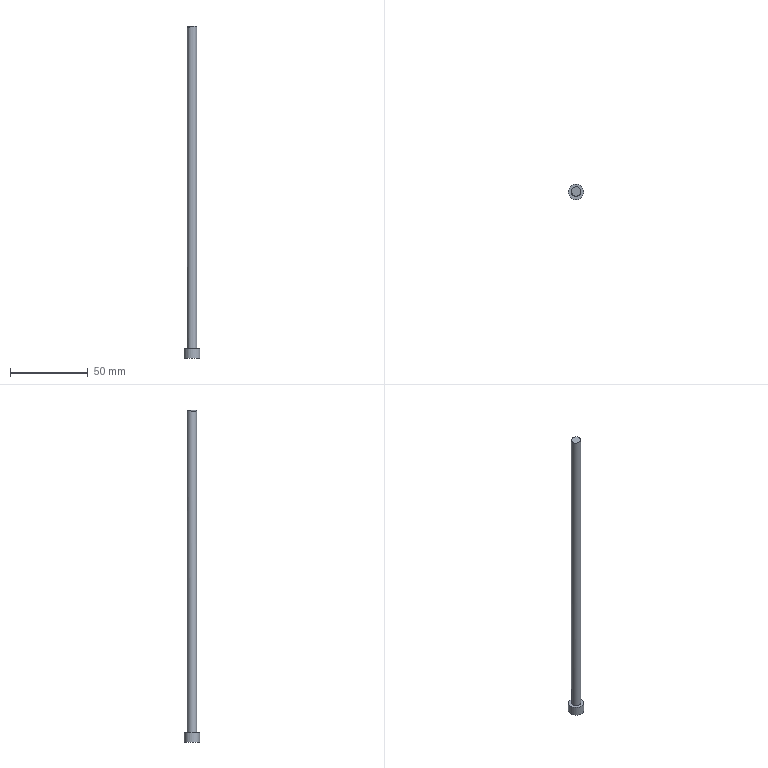Part | NX | features DDZ6.00 2 | 1 solid | 5 faces | box 10 x 10 x 214.007 mm | volume 6341 mm3 | cylinder 2 | plane 2 | sphere 1 | commonest cylinder face diameters 6 x1 10 x1
STEP:
#1=CARTESIAN_POINT('',(-27.91,-12.97,-204.5));
#2=VERTEX_POINT('',#1);
#3=CARTESIAN_POINT('',(-30.91,-12.97,-204.5));
#4=DIRECTION('',(0.,0.,1.));
#5=DIRECTION('',(1.,0.,0.));
#6=AXIS2_PLACEMENT_3D('',#3,#4,#5);
#7=CIRCLE('',#6,3.);
#8=EDGE_CURVE('',#2,#2,#7,.F.);
#9=ORIENTED_EDGE('',*,*,#8,.F.);
#10=EDGE_LOOP('',(#9));
#11=FACE_BOUND('',#10,.T.);
#12=CARTESIAN_POINT('',(-33.046,-15.077,2.797));
#13=VERTEX_POINT('',#12);
#14=CARTESIAN_POINT('',(-30.927,-16.293,2.98));
#15=CARTESIAN_POINT('',(-33.278,-15.308,2.76));
#16=CARTESIAN_POINT('',(-34.236,-12.935,2.764));
#17=CARTESIAN_POINT('',(-33.236,-10.599,2.989));
#18=CARTESIAN_POINT('',(-30.891,-9.647,3.3));
#19=CARTESIAN_POINT('',(-28.544,-10.632,3.519));
#20=CARTESIAN_POINT('',(-27.583,-13.,3.515));
#21=CARTESIAN_POINT('',(-28.583,-15.341,3.291));
#22=CARTESIAN_POINT('',(-30.927,-16.293,2.98));
#23=CARTESIAN_POINT('',(-33.278,-15.308,2.76));
#24=CARTESIAN_POINT('',(-34.236,-12.935,2.764));
#25=B_SPLINE_CURVE_WITH_KNOTS('',3,(#14,#15,#16,#17,#18,#19,#20,#21,#22,#23,#24),.UNSPECIFIED.,.T.,.F.,(1,1,1,1,1,1,1,1,1,1,1,1,1,1,1),(-0.007061,-0.004707,-0.002354,0.,0.002354,0.004707,0.007061,0.009414,0.01177,0.01412,0.01648,0.01883,0.02118,0.02354,0.02589),.UNSPECIFIED.);
#26=EDGE_CURVE('',#13,#13,#25,.T.);
#27=ORIENTED_EDGE('',*,*,#26,.T.);
#28=EDGE_LOOP('',(#27));
#29=FACE_BOUND('',#28,.T.);
#30=CARTESIAN_POINT('',(-30.91,-12.97,-210.5));
#31=DIRECTION('',(0.,0.,1.));
#32=DIRECTION('',(1.,0.,0.));
#33=AXIS2_PLACEMENT_3D('',#30,#31,#32);
#34=CYLINDRICAL_SURFACE('',#33,3.);
#35=ADVANCED_FACE('',(#11,#29),#34,.T.);
#36=ORIENTED_EDGE('',*,*,#8,.T.);
#37=EDGE_LOOP('',(#36));
#38=FACE_BOUND('',#37,.T.);
#39=CARTESIAN_POINT('',(-25.91,-12.97,-204.5));
#40=VERTEX_POINT('',#39);
#41=CARTESIAN_POINT('',(-30.91,-12.97,-204.5));
#42=DIRECTION('',(0.,0.,-1.));
#43=DIRECTION('',(1.,0.,0.));
#44=AXIS2_PLACEMENT_3D('',#41,#42,#43);
#45=CIRCLE('',#44,5.);
#46=EDGE_CURVE('',#40,#40,#45,.T.);
#47=ORIENTED_EDGE('',*,*,#46,.F.);
#48=EDGE_LOOP('',(#47));
#49=FACE_BOUND('',#48,.T.);
#50=CARTESIAN_POINT('',(-30.91,-12.97,-204.5));
#51=DIRECTION('',(0.,0.,1.));
#52=DIRECTION('',(1.,0.,0.));
#53=AXIS2_PLACEMENT_3D('',#50,#51,#52);
#54=PLANE('',#53);
#55=ADVANCED_FACE('',(#38,#49),#54,.T.);
#56=ORIENTED_EDGE('',*,*,#46,.T.);
#57=EDGE_LOOP('',(#56));
#58=FACE_BOUND('',#57,.T.);
#59=CARTESIAN_POINT('',(-25.91,-12.97,-210.5));
#60=VERTEX_POINT('',#59);
#61=CARTESIAN_POINT('',(-30.91,-12.97,-210.5));
#62=DIRECTION('',(0.,0.,1.));
#63=DIRECTION('',(1.,0.,0.));
#64=AXIS2_PLACEMENT_3D('',#61,#62,#63);
#65=CIRCLE('',#64,5.);
#66=EDGE_CURVE('',#60,#60,#65,.T.);
#67=ORIENTED_EDGE('',*,*,#66,.T.);
#68=EDGE_LOOP('',(#67));
#69=FACE_BOUND('',#68,.T.);
#70=CARTESIAN_POINT('',(-30.91,-12.97,-210.5));
#71=DIRECTION('',(0.,0.,1.));
#72=DIRECTION('',(1.,0.,0.));
#73=AXIS2_PLACEMENT_3D('',#70,#71,#72);
#74=CYLINDRICAL_SURFACE('',#73,5.);
#75=ADVANCED_FACE('',(#58,#69),#74,.T.);
#76=ORIENTED_EDGE('',*,*,#66,.F.);
#77=EDGE_LOOP('',(#76));
#78=FACE_BOUND('',#77,.T.);
#79=CARTESIAN_POINT('',(-30.91,-12.97,-210.5));
#80=DIRECTION('',(0.,0.,-1.));
#81=DIRECTION('',(-1.,0.,0.));
#82=AXIS2_PLACEMENT_3D('',#79,#80,#81);
#83=PLANE('',#82);
#84=ADVANCED_FACE('',(#78),#83,.T.);
#85=ORIENTED_EDGE('',*,*,#26,.F.);
#86=EDGE_LOOP('',(#85));
#87=FACE_BOUND('',#86,.T.);
#88=CARTESIAN_POINT('',(0.,0.,-269.66));
#89=DIRECTION('',(0.,0.,-1.));
#90=DIRECTION('',(1.,0.,0.));
#91=AXIS2_PLACEMENT_3D('',#88,#89,#90);
#92=SPHERICAL_SURFACE('',#91,274.868);
#93=ADVANCED_FACE('',(#87),#92,.T.);
#94=CLOSED_SHELL('',(#35,#55,#75,#84,#93));
#95=MANIFOLD_SOLID_BREP('',#94);
#96=(LENGTH_UNIT()NAMED_UNIT(*)SI_UNIT(.MILLI.,.METRE.));
#97=UNCERTAINTY_MEASURE_WITH_UNIT(LENGTH_MEASURE(0.0508),#96,'','');
#98=(NAMED_UNIT(*)PLANE_ANGLE_UNIT()SI_UNIT($,.RADIAN.));
#99=(NAMED_UNIT(*)SI_UNIT($,.STERADIAN.)SOLID_ANGLE_UNIT());
#100=(GEOMETRIC_REPRESENTATION_CONTEXT(3)GLOBAL_UNCERTAINTY_ASSIGNED_CONTEXT((#97))GLOBAL_UNIT_ASSIGNED_CONTEXT((#96,#98,#99))REPRESENTATION_CONTEXT('',''));
#101=ADVANCED_BREP_SHAPE_REPRESENTATION('',(#95),#100);